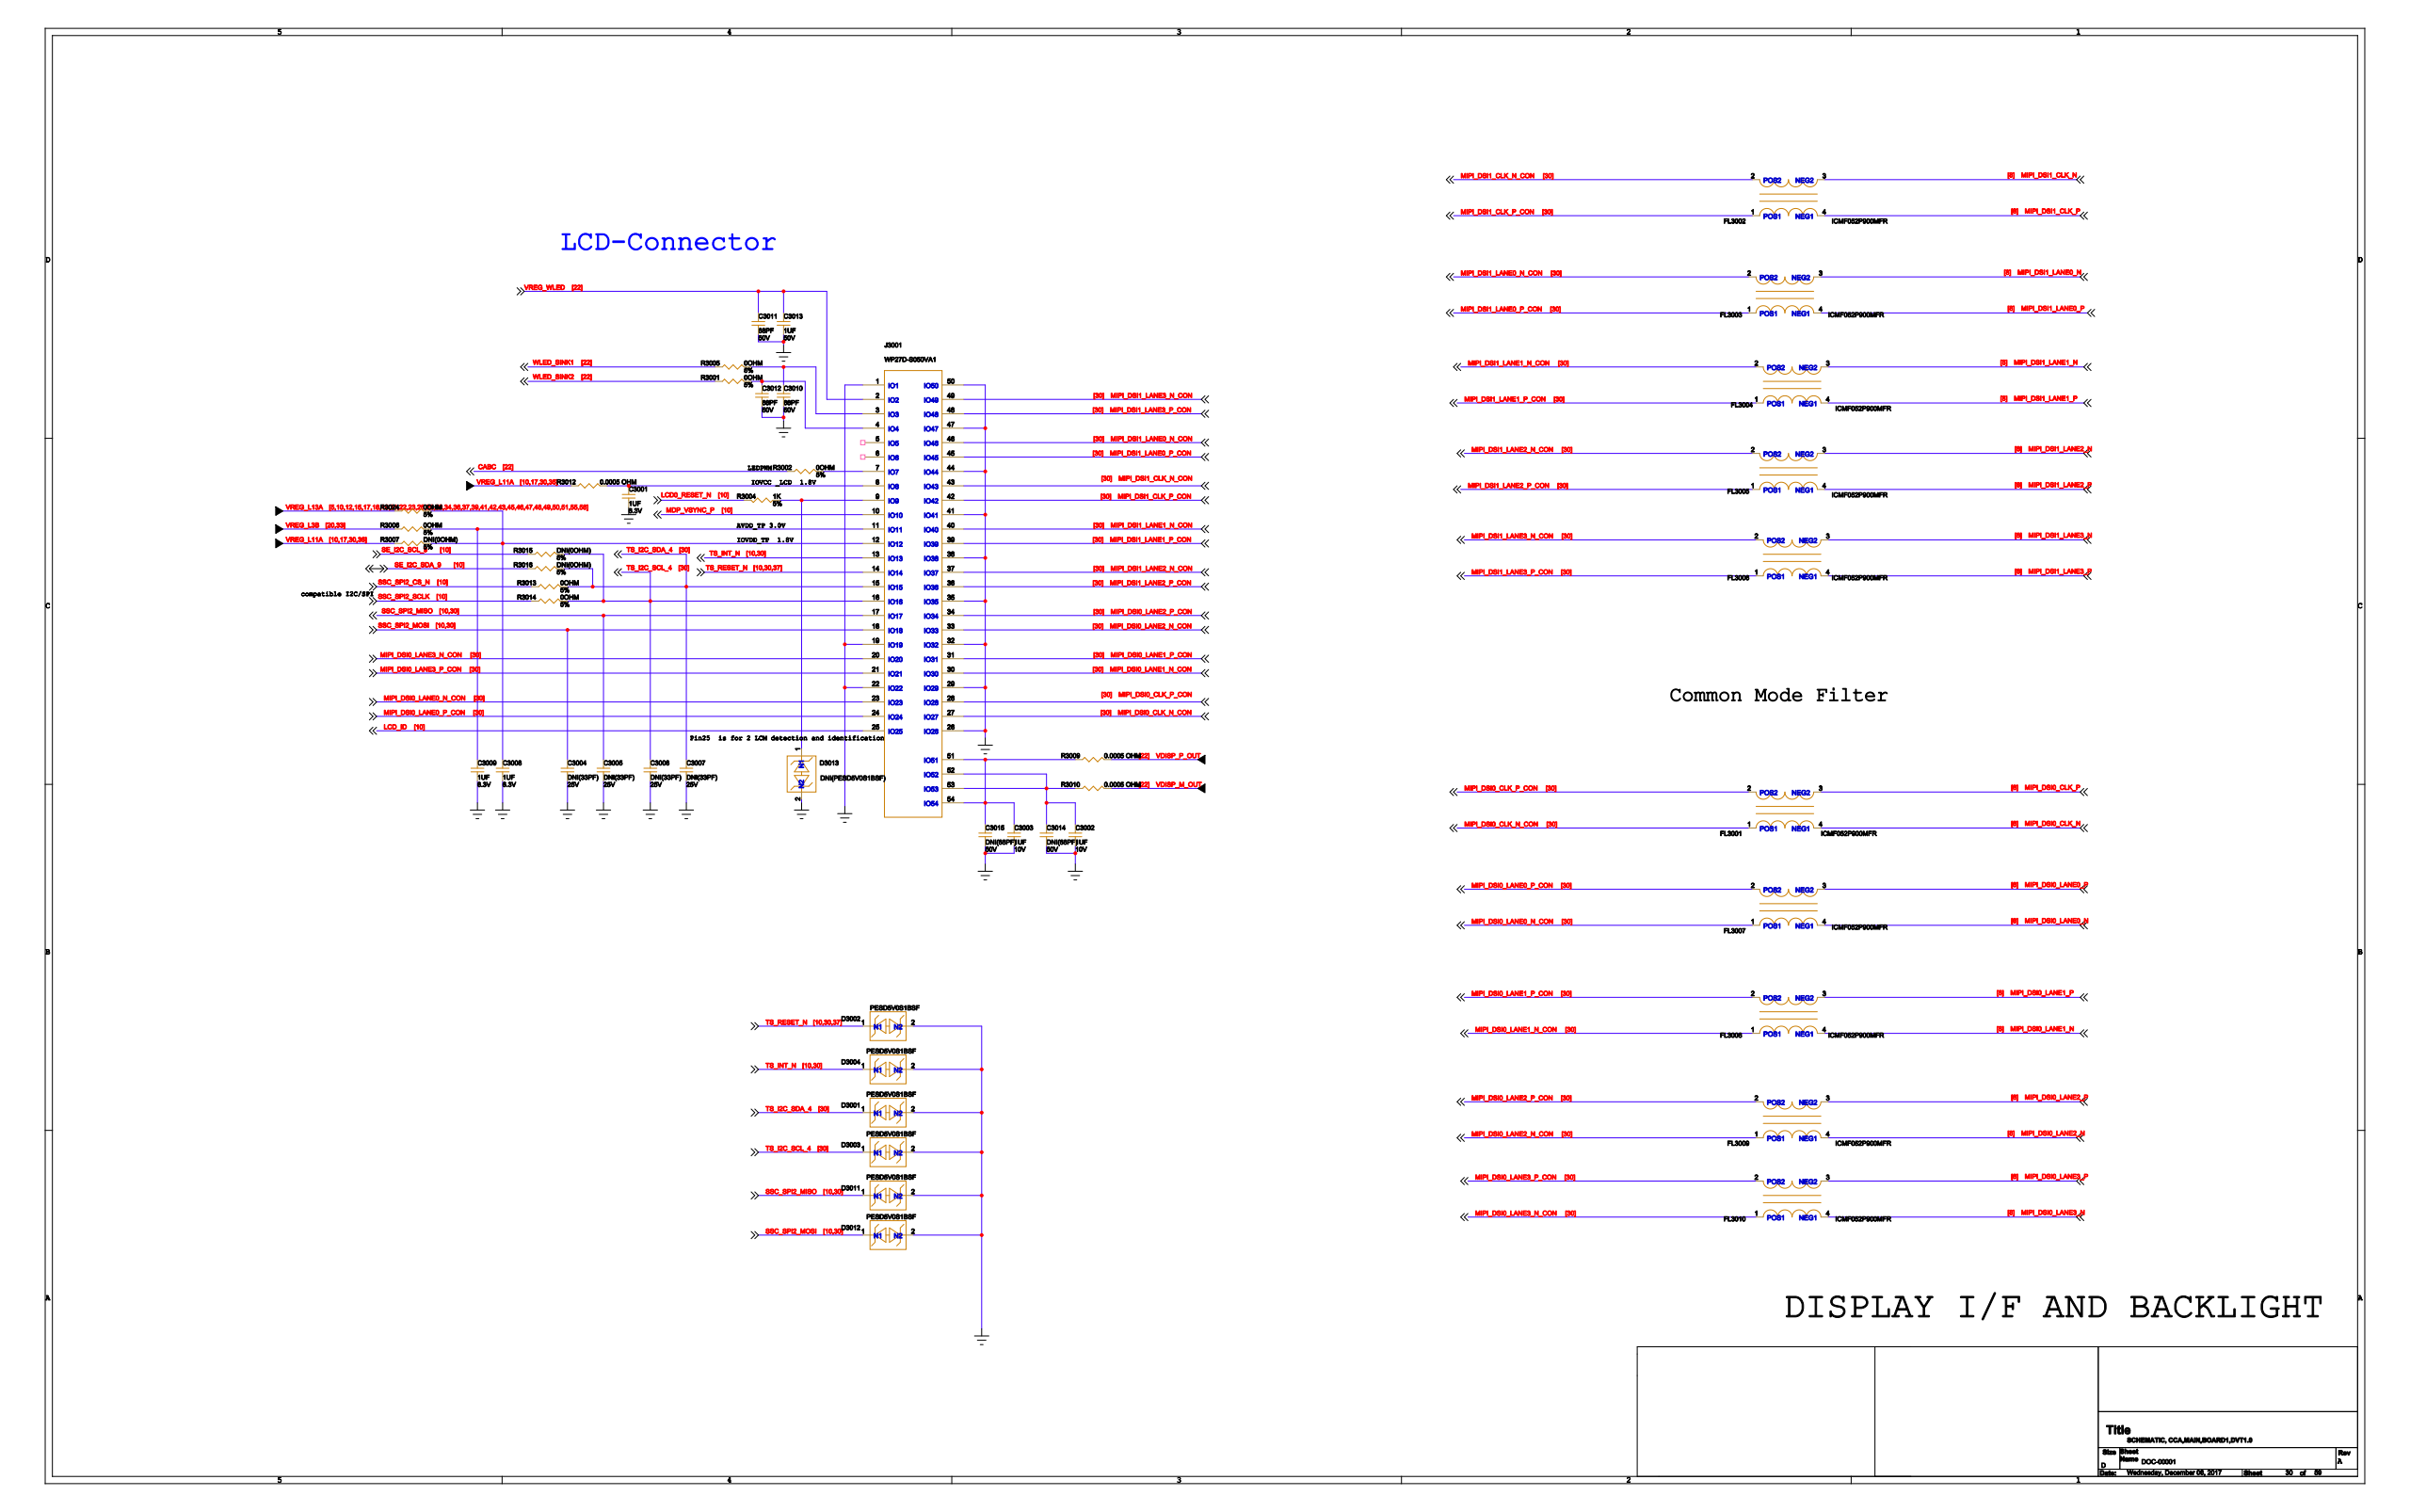Circuit board | KiCad | 1657 parts | 1365 nets | one sheet of the schematic
Parts on this sheet (reference | value | footprint):
C3001
C3002
C3003
C3004
C3005
C3006
C3007
C3008
C3009
C3010
C3011
C3012
C3013
C3014
C3015
D3001
D3002
D3003
D3004
D3011
D3012
D3013
FL3001
FL3002
FL3003
FL3004
FL3005
FL3006
FL3007
FL3008
FL3009
FL3010
J3001
R3001
R3002
R3004
R3005
R3006
R3007
R3009
R3010
R3012
R3013
R3014
R3015
R3016
R3024
Nets of these parts (net: part-pin ...):
GND: C3001-2 C3002-2 C3003-2 C3004-2 C3005-2 C3006-2 C3007-2 C3008-2 C3009-2 C3010-2 C3011-2 C3012-2 C3013-2 C3014-2 C3015-2 D3001-2 D3002-2 D3003-2 D3004-2 D3011-2 D3012-2 D3013-2 J3001-1 J3001-19 J3001-22 J3001-26 J3001-29 J3001-32 J3001-35 J3001-38 J3001-41 J3001-44 J3001-47 J3001-50
VREG_L13A: R3024-2
I1_LANE2_P_CON: FL3005-1 J3001-36
I1_LANE2_N_CON: FL3005-2 J3001-37
I_DSI1_LANE2_N: FL3005-3
I_DSI1_LANE2_P: FL3005-4
N19768603: D3013-1 R3004-2 J3001-9
TS_INT_N: D3004-1 J3001-13
N19768853: R3002-1 J3001-7
CABC: R3002-2
LCD0_RESET_N: R3004-1
TS_I2C_SCL_4: C3006-1 D3003-1 R3014-1 R3015-1 J3001-16
SSC_SPI2_SCLK: R3014-2
N19768457: C3008-1 R3007-1 R3024-1 J3001-12
VREG_L11A: R3007-2 R3012-2
N19768619: C3003-1 C3015-1 R3009-2 J3001-51 J3001-54
I1_LANE1_P_CON: FL3004-1 J3001-39
I1_LANE1_N_CON: FL3004-2 J3001-40
I_DSI1_LANE1_N: FL3004-3
I_DSI1_LANE1_P: FL3004-4
I1_LANE3_P_CON: FL3006-1 J3001-48
I1_LANE3_N_CON: FL3006-2 J3001-49
I_DSI1_LANE3_N: FL3006-3
I_DSI1_LANE3_P: FL3006-4
TS_RESET_N: D3002-1 J3001-14
TS_I2C_SDA_4: C3007-1 D3001-1 R3013-1 R3016-1 J3001-15
SE_I2C_SDA_9: R3016-2
N19768601: C3001-1 R3012-1 J3001-8
I1_LANE0_P_CON: FL3003-1 J3001-45
I1_LANE0_N_CON: FL3003-2 J3001-46
I_DSI1_LANE0_N: FL3003-3
I_DSI1_LANE0_P: FL3003-4
N19768791: C3012-1 R3001-1 J3001-4
I0_LANE2_N_CON: FL3009-1 J3001-33
I0_LANE2_P_CON: FL3009-2 J3001-34
I_DSI0_LANE2_P: FL3009-3
I_DSI0_LANE2_N: FL3009-4
N19768625: C3002-1 C3014-1 R3010-2 J3001-52 J3001-53
DSI1_CLK_P_CON: FL3002-1 J3001-42
DSI1_CLK_N_CON: FL3002-2 J3001-43
IPI_DSI1_CLK_N: FL3002-3
IPI_DSI1_CLK_P: FL3002-4
N19768893: C3009-1 R3006-1 J3001-11
SE_I2C_SCL_9: R3015-2
SSC_SPI2_CS_N: R3013-2
SSC_SPI2_MISO: C3005-1 D3011-1 J3001-17
I0_LANE3_N_CON: FL3010-1 J3001-20
I0_LANE3_P_CON: FL3010-2 J3001-21
I_DSI0_LANE3_P: FL3010-3
I_DSI0_LANE3_N: FL3010-4
I0_LANE1_N_CON: FL3008-1 J3001-30
I0_LANE1_P_CON: FL3008-2 J3001-31
I_DSI0_LANE1_P: FL3008-3
I_DSI0_LANE1_N: FL3008-4
SSC_SPI2_MOSI: C3004-1 D3012-1 J3001-18
LCD_ID: J3001-25
IPI_DSI0_CLK_N: FL3001-4
IPI_DSI0_CLK_P: FL3001-3
I_DSI0_LANE0_N: FL3007-4
I_DSI0_LANE0_P: FL3007-3
MDP_VSYNC_P: J3001-10
VDISP_P_OUT: R3009-1
VDISP_M_OUT: R3010-1
I0_LANE0_N_CON: FL3007-1 J3001-23
I0_LANE0_P_CON: FL3007-2 J3001-24
VREG_L3B: R3006-2
WLED_SINK2: R3001-2
VREG_WLED: C3011-1 C3013-1 J3001-2
N19768795: C3010-1 R3005-1 J3001-3
DSI0_CLK_N_CON: FL3001-1 J3001-27
DSI0_CLK_P_CON: FL3001-2 J3001-28
WLED_SINK1: R3005-2